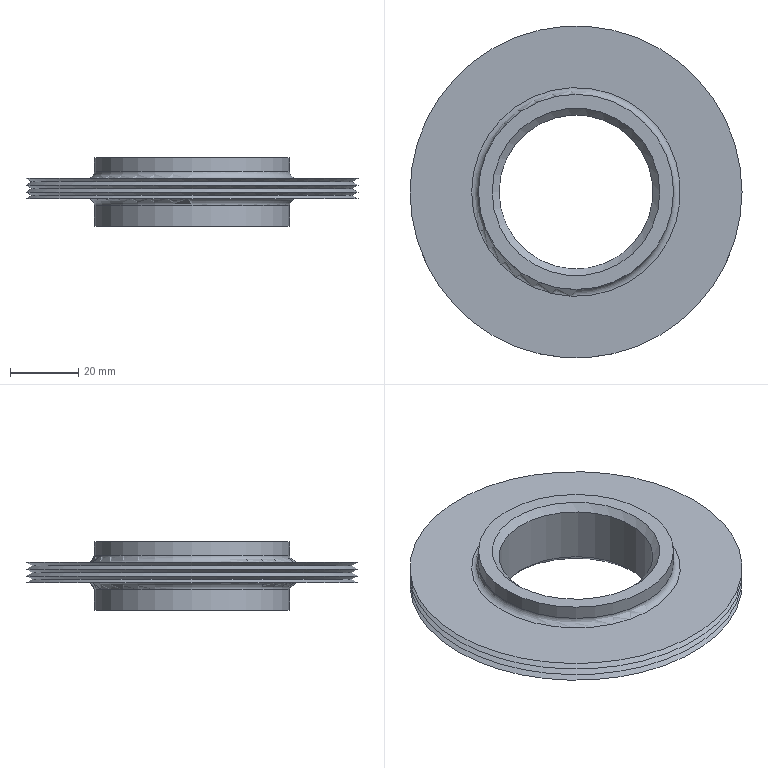Part | NX | features DATUM_CSYS 2, SKETCH 1, SWP104 1 | 1 solid | 17 faces | box 97 x 97 x 20 mm | volume 46420 mm3 | cone 8 | plane 4 | cylinder 3 | torus 2 | commonest cylinder face diameters 57 x2 45 x1
STEP:
#1=CARTESIAN_POINT('',(-48.5,0.,8.));
#2=VERTEX_POINT('',#1);
#3=CARTESIAN_POINT('',(0.,0.,8.));
#4=DIRECTION('',(0.,0.,-1.));
#5=DIRECTION('',(-1.,0.,0.));
#6=AXIS2_PLACEMENT_3D('',#3,#4,#5);
#7=CIRCLE('',#6,48.5);
#8=EDGE_CURVE('',#2,#2,#7,.T.);
#9=ORIENTED_EDGE('',*,*,#8,.F.);
#10=EDGE_LOOP('',(#9));
#11=FACE_BOUND('',#10,.T.);
#12=CARTESIAN_POINT('',(-46.768,0.,9.));
#13=VERTEX_POINT('',#12);
#14=CARTESIAN_POINT('',(0.,0.,9.));
#15=DIRECTION('',(0.,0.,-1.));
#16=DIRECTION('',(-1.,0.,0.));
#17=AXIS2_PLACEMENT_3D('',#14,#15,#16);
#18=CIRCLE('',#17,46.768);
#19=EDGE_CURVE('',#13,#13,#18,.T.);
#20=ORIENTED_EDGE('',*,*,#19,.T.);
#21=EDGE_LOOP('',(#20));
#22=FACE_BOUND('',#21,.T.);
#23=CARTESIAN_POINT('',(0.,0.,9.));
#24=DIRECTION('',(0.,0.,-1.));
#25=DIRECTION('',(-1.,0.,0.));
#26=AXIS2_PLACEMENT_3D('',#23,#24,#25);
#27=CONICAL_SURFACE('',#26,46.768,1.047);
#28=ADVANCED_FACE('',(#11,#22),#27,.T.);
#29=CARTESIAN_POINT('',(-30.5,0.,8.));
#30=VERTEX_POINT('',#29);
#31=CARTESIAN_POINT('',(0.,0.,8.));
#32=DIRECTION('',(0.,0.,-1.));
#33=DIRECTION('',(-1.,0.,0.));
#34=AXIS2_PLACEMENT_3D('',#31,#32,#33);
#35=CIRCLE('',#34,30.5);
#36=EDGE_CURVE('',#30,#30,#35,.T.);
#37=ORIENTED_EDGE('',*,*,#36,.F.);
#38=EDGE_LOOP('',(#37));
#39=FACE_BOUND('',#38,.T.);
#40=ORIENTED_EDGE('',*,*,#8,.T.);
#41=EDGE_LOOP('',(#40));
#42=FACE_BOUND('',#41,.T.);
#43=CARTESIAN_POINT('',(0.,-48.5,8.));
#44=DIRECTION('',(0.,0.,1.));
#45=DIRECTION('',(1.,0.,0.));
#46=AXIS2_PLACEMENT_3D('',#43,#44,#45);
#47=PLANE('',#46);
#48=ADVANCED_FACE('',(#39,#42),#47,.F.);
#49=CARTESIAN_POINT('',(-28.5,0.,6.));
#50=VERTEX_POINT('',#49);
#51=CARTESIAN_POINT('',(0.,0.,6.));
#52=DIRECTION('',(0.,0.,-1.));
#53=DIRECTION('',(-1.,0.,0.));
#54=AXIS2_PLACEMENT_3D('',#51,#52,#53);
#55=CIRCLE('',#54,28.5);
#56=EDGE_CURVE('',#50,#50,#55,.T.);
#57=ORIENTED_EDGE('',*,*,#56,.F.);
#58=EDGE_LOOP('',(#57));
#59=FACE_BOUND('',#58,.T.);
#60=ORIENTED_EDGE('',*,*,#36,.T.);
#61=EDGE_LOOP('',(#60));
#62=FACE_BOUND('',#61,.T.);
#63=CARTESIAN_POINT('',(0.,0.,6.));
#64=DIRECTION('',(0.,0.,-1.));
#65=DIRECTION('',(-1.,0.,0.));
#66=AXIS2_PLACEMENT_3D('',#63,#64,#65);
#67=TOROIDAL_SURFACE('',#66,30.5,2.);
#68=ADVANCED_FACE('',(#59,#62),#67,.F.);
#69=CARTESIAN_POINT('',(-28.5,0.,0.));
#70=VERTEX_POINT('',#69);
#71=CARTESIAN_POINT('',(0.,0.,0.));
#72=DIRECTION('',(0.,0.,-1.));
#73=DIRECTION('',(-1.,0.,0.));
#74=AXIS2_PLACEMENT_3D('',#71,#72,#73);
#75=CIRCLE('',#74,28.5);
#76=EDGE_CURVE('',#70,#70,#75,.T.);
#77=ORIENTED_EDGE('',*,*,#76,.F.);
#78=EDGE_LOOP('',(#77));
#79=FACE_BOUND('',#78,.T.);
#80=ORIENTED_EDGE('',*,*,#56,.T.);
#81=EDGE_LOOP('',(#80));
#82=FACE_BOUND('',#81,.T.);
#83=CARTESIAN_POINT('',(0.,0.,0.));
#84=DIRECTION('',(0.,0.,-1.));
#85=DIRECTION('',(-1.,0.,0.));
#86=AXIS2_PLACEMENT_3D('',#83,#84,#85);
#87=CYLINDRICAL_SURFACE('',#86,28.5);
#88=ADVANCED_FACE('',(#79,#82),#87,.T.);
#89=CARTESIAN_POINT('',(-24.5,0.,0.));
#90=VERTEX_POINT('',#89);
#91=CARTESIAN_POINT('',(0.,0.,0.));
#92=DIRECTION('',(0.,0.,-1.));
#93=DIRECTION('',(-1.,0.,0.));
#94=AXIS2_PLACEMENT_3D('',#91,#92,#93);
#95=CIRCLE('',#94,24.5);
#96=EDGE_CURVE('',#90,#90,#95,.T.);
#97=ORIENTED_EDGE('',*,*,#96,.F.);
#98=EDGE_LOOP('',(#97));
#99=FACE_BOUND('',#98,.T.);
#100=ORIENTED_EDGE('',*,*,#76,.T.);
#101=EDGE_LOOP('',(#100));
#102=FACE_BOUND('',#101,.T.);
#103=CARTESIAN_POINT('',(0.,-28.5,0.));
#104=DIRECTION('',(0.,0.,1.));
#105=DIRECTION('',(1.,0.,0.));
#106=AXIS2_PLACEMENT_3D('',#103,#104,#105);
#107=PLANE('',#106);
#108=ADVANCED_FACE('',(#99,#102),#107,.F.);
#109=CARTESIAN_POINT('',(-22.5,0.,2.));
#110=VERTEX_POINT('',#109);
#111=CARTESIAN_POINT('',(0.,0.,2.));
#112=DIRECTION('',(0.,0.,-1.));
#113=DIRECTION('',(-1.,0.,0.));
#114=AXIS2_PLACEMENT_3D('',#111,#112,#113);
#115=CIRCLE('',#114,22.5);
#116=EDGE_CURVE('',#110,#110,#115,.T.);
#117=ORIENTED_EDGE('',*,*,#116,.F.);
#118=EDGE_LOOP('',(#117));
#119=FACE_BOUND('',#118,.T.);
#120=ORIENTED_EDGE('',*,*,#96,.T.);
#121=EDGE_LOOP('',(#120));
#122=FACE_BOUND('',#121,.T.);
#123=CARTESIAN_POINT('',(0.,0.,0.));
#124=DIRECTION('',(0.,0.,-1.));
#125=DIRECTION('',(-1.,0.,0.));
#126=AXIS2_PLACEMENT_3D('',#123,#124,#125);
#127=CONICAL_SURFACE('',#126,24.5,0.7854);
#128=ADVANCED_FACE('',(#119,#122),#127,.F.);
#129=CARTESIAN_POINT('',(-22.5,0.,18.));
#130=VERTEX_POINT('',#129);
#131=CARTESIAN_POINT('',(0.,0.,18.));
#132=DIRECTION('',(0.,0.,-1.));
#133=DIRECTION('',(-1.,0.,0.));
#134=AXIS2_PLACEMENT_3D('',#131,#132,#133);
#135=CIRCLE('',#134,22.5);
#136=EDGE_CURVE('',#130,#130,#135,.T.);
#137=ORIENTED_EDGE('',*,*,#136,.F.);
#138=EDGE_LOOP('',(#137));
#139=FACE_BOUND('',#138,.T.);
#140=ORIENTED_EDGE('',*,*,#116,.T.);
#141=EDGE_LOOP('',(#140));
#142=FACE_BOUND('',#141,.T.);
#143=CARTESIAN_POINT('',(0.,0.,0.));
#144=DIRECTION('',(0.,0.,-1.));
#145=DIRECTION('',(-1.,0.,0.));
#146=AXIS2_PLACEMENT_3D('',#143,#144,#145);
#147=CYLINDRICAL_SURFACE('',#146,22.5);
#148=ADVANCED_FACE('',(#139,#142),#147,.F.);
#149=CARTESIAN_POINT('',(-24.5,0.,20.));
#150=VERTEX_POINT('',#149);
#151=CARTESIAN_POINT('',(0.,0.,20.));
#152=DIRECTION('',(0.,0.,-1.));
#153=DIRECTION('',(-1.,0.,0.));
#154=AXIS2_PLACEMENT_3D('',#151,#152,#153);
#155=CIRCLE('',#154,24.5);
#156=EDGE_CURVE('',#150,#150,#155,.T.);
#157=ORIENTED_EDGE('',*,*,#156,.F.);
#158=EDGE_LOOP('',(#157));
#159=FACE_BOUND('',#158,.T.);
#160=ORIENTED_EDGE('',*,*,#136,.T.);
#161=EDGE_LOOP('',(#160));
#162=FACE_BOUND('',#161,.T.);
#163=CARTESIAN_POINT('',(0.,0.,18.));
#164=DIRECTION('',(0.,0.,1.));
#165=DIRECTION('',(1.,0.,0.));
#166=AXIS2_PLACEMENT_3D('',#163,#164,#165);
#167=CONICAL_SURFACE('',#166,22.5,0.7854);
#168=ADVANCED_FACE('',(#159,#162),#167,.F.);
#169=CARTESIAN_POINT('',(-28.5,0.,20.));
#170=VERTEX_POINT('',#169);
#171=CARTESIAN_POINT('',(0.,0.,20.));
#172=DIRECTION('',(0.,0.,-1.));
#173=DIRECTION('',(-1.,0.,0.));
#174=AXIS2_PLACEMENT_3D('',#171,#172,#173);
#175=CIRCLE('',#174,28.5);
#176=EDGE_CURVE('',#170,#170,#175,.T.);
#177=ORIENTED_EDGE('',*,*,#176,.F.);
#178=EDGE_LOOP('',(#177));
#179=FACE_BOUND('',#178,.T.);
#180=ORIENTED_EDGE('',*,*,#156,.T.);
#181=EDGE_LOOP('',(#180));
#182=FACE_BOUND('',#181,.T.);
#183=CARTESIAN_POINT('',(0.,-24.5,20.));
#184=DIRECTION('',(0.,0.,-1.));
#185=DIRECTION('',(-1.,0.,0.));
#186=AXIS2_PLACEMENT_3D('',#183,#184,#185);
#187=PLANE('',#186);
#188=ADVANCED_FACE('',(#179,#182),#187,.F.);
#189=CARTESIAN_POINT('',(-28.5,0.,16.));
#190=VERTEX_POINT('',#189);
#191=CARTESIAN_POINT('',(0.,0.,16.));
#192=DIRECTION('',(0.,0.,-1.));
#193=DIRECTION('',(-1.,0.,0.));
#194=AXIS2_PLACEMENT_3D('',#191,#192,#193);
#195=CIRCLE('',#194,28.5);
#196=EDGE_CURVE('',#190,#190,#195,.T.);
#197=ORIENTED_EDGE('',*,*,#196,.F.);
#198=EDGE_LOOP('',(#197));
#199=FACE_BOUND('',#198,.T.);
#200=ORIENTED_EDGE('',*,*,#176,.T.);
#201=EDGE_LOOP('',(#200));
#202=FACE_BOUND('',#201,.T.);
#203=CARTESIAN_POINT('',(0.,0.,0.));
#204=DIRECTION('',(0.,0.,-1.));
#205=DIRECTION('',(-1.,0.,0.));
#206=AXIS2_PLACEMENT_3D('',#203,#204,#205);
#207=CYLINDRICAL_SURFACE('',#206,28.5);
#208=ADVANCED_FACE('',(#199,#202),#207,.T.);
#209=CARTESIAN_POINT('',(-30.5,0.,14.));
#210=VERTEX_POINT('',#209);
#211=CARTESIAN_POINT('',(0.,0.,14.));
#212=DIRECTION('',(0.,0.,-1.));
#213=DIRECTION('',(-1.,0.,0.));
#214=AXIS2_PLACEMENT_3D('',#211,#212,#213);
#215=CIRCLE('',#214,30.5);
#216=EDGE_CURVE('',#210,#210,#215,.T.);
#217=ORIENTED_EDGE('',*,*,#216,.F.);
#218=EDGE_LOOP('',(#217));
#219=FACE_BOUND('',#218,.T.);
#220=ORIENTED_EDGE('',*,*,#196,.T.);
#221=EDGE_LOOP('',(#220));
#222=FACE_BOUND('',#221,.T.);
#223=CARTESIAN_POINT('',(0.,0.,16.));
#224=DIRECTION('',(0.,0.,-1.));
#225=DIRECTION('',(-1.,0.,0.));
#226=AXIS2_PLACEMENT_3D('',#223,#224,#225);
#227=TOROIDAL_SURFACE('',#226,30.5,2.);
#228=ADVANCED_FACE('',(#219,#222),#227,.F.);
#229=CARTESIAN_POINT('',(-48.5,0.,14.));
#230=VERTEX_POINT('',#229);
#231=CARTESIAN_POINT('',(0.,0.,14.));
#232=DIRECTION('',(0.,0.,-1.));
#233=DIRECTION('',(-1.,0.,0.));
#234=AXIS2_PLACEMENT_3D('',#231,#232,#233);
#235=CIRCLE('',#234,48.5);
#236=EDGE_CURVE('',#230,#230,#235,.T.);
#237=ORIENTED_EDGE('',*,*,#236,.F.);
#238=EDGE_LOOP('',(#237));
#239=FACE_BOUND('',#238,.T.);
#240=ORIENTED_EDGE('',*,*,#216,.T.);
#241=EDGE_LOOP('',(#240));
#242=FACE_BOUND('',#241,.T.);
#243=CARTESIAN_POINT('',(0.,-30.5,14.));
#244=DIRECTION('',(0.,0.,-1.));
#245=DIRECTION('',(-1.,0.,0.));
#246=AXIS2_PLACEMENT_3D('',#243,#244,#245);
#247=PLANE('',#246);
#248=ADVANCED_FACE('',(#239,#242),#247,.F.);
#249=CARTESIAN_POINT('',(-46.768,0.,13.));
#250=VERTEX_POINT('',#249);
#251=CARTESIAN_POINT('',(0.,0.,13.));
#252=DIRECTION('',(0.,0.,-1.));
#253=DIRECTION('',(-1.,0.,0.));
#254=AXIS2_PLACEMENT_3D('',#251,#252,#253);
#255=CIRCLE('',#254,46.768);
#256=EDGE_CURVE('',#250,#250,#255,.T.);
#257=ORIENTED_EDGE('',*,*,#256,.F.);
#258=EDGE_LOOP('',(#257));
#259=FACE_BOUND('',#258,.T.);
#260=ORIENTED_EDGE('',*,*,#236,.T.);
#261=EDGE_LOOP('',(#260));
#262=FACE_BOUND('',#261,.T.);
#263=CARTESIAN_POINT('',(0.,0.,14.));
#264=DIRECTION('',(0.,0.,1.));
#265=DIRECTION('',(1.,0.,0.));
#266=AXIS2_PLACEMENT_3D('',#263,#264,#265);
#267=CONICAL_SURFACE('',#266,48.5,1.047);
#268=ADVANCED_FACE('',(#259,#262),#267,.T.);
#269=CARTESIAN_POINT('',(-48.5,0.,12.));
#270=VERTEX_POINT('',#269);
#271=CARTESIAN_POINT('',(0.,0.,12.));
#272=DIRECTION('',(0.,0.,-1.));
#273=DIRECTION('',(-1.,0.,0.));
#274=AXIS2_PLACEMENT_3D('',#271,#272,#273);
#275=CIRCLE('',#274,48.5);
#276=EDGE_CURVE('',#270,#270,#275,.T.);
#277=ORIENTED_EDGE('',*,*,#276,.F.);
#278=EDGE_LOOP('',(#277));
#279=FACE_BOUND('',#278,.T.);
#280=ORIENTED_EDGE('',*,*,#256,.T.);
#281=EDGE_LOOP('',(#280));
#282=FACE_BOUND('',#281,.T.);
#283=CARTESIAN_POINT('',(0.,0.,13.));
#284=DIRECTION('',(0.,0.,-1.));
#285=DIRECTION('',(-1.,0.,0.));
#286=AXIS2_PLACEMENT_3D('',#283,#284,#285);
#287=CONICAL_SURFACE('',#286,46.768,1.047);
#288=ADVANCED_FACE('',(#279,#282),#287,.T.);
#289=CARTESIAN_POINT('',(-46.768,0.,11.));
#290=VERTEX_POINT('',#289);
#291=CARTESIAN_POINT('',(0.,0.,11.));
#292=DIRECTION('',(0.,0.,-1.));
#293=DIRECTION('',(-1.,0.,0.));
#294=AXIS2_PLACEMENT_3D('',#291,#292,#293);
#295=CIRCLE('',#294,46.768);
#296=EDGE_CURVE('',#290,#290,#295,.T.);
#297=ORIENTED_EDGE('',*,*,#296,.F.);
#298=EDGE_LOOP('',(#297));
#299=FACE_BOUND('',#298,.T.);
#300=ORIENTED_EDGE('',*,*,#276,.T.);
#301=EDGE_LOOP('',(#300));
#302=FACE_BOUND('',#301,.T.);
#303=CARTESIAN_POINT('',(0.,0.,12.));
#304=DIRECTION('',(0.,0.,1.));
#305=DIRECTION('',(1.,0.,0.));
#306=AXIS2_PLACEMENT_3D('',#303,#304,#305);
#307=CONICAL_SURFACE('',#306,48.5,1.047);
#308=ADVANCED_FACE('',(#299,#302),#307,.T.);
#309=CARTESIAN_POINT('',(-48.5,0.,10.));
#310=VERTEX_POINT('',#309);
#311=CARTESIAN_POINT('',(0.,0.,10.));
#312=DIRECTION('',(0.,0.,-1.));
#313=DIRECTION('',(-1.,0.,0.));
#314=AXIS2_PLACEMENT_3D('',#311,#312,#313);
#315=CIRCLE('',#314,48.5);
#316=EDGE_CURVE('',#310,#310,#315,.T.);
#317=ORIENTED_EDGE('',*,*,#316,.F.);
#318=EDGE_LOOP('',(#317));
#319=FACE_BOUND('',#318,.T.);
#320=ORIENTED_EDGE('',*,*,#296,.T.);
#321=EDGE_LOOP('',(#320));
#322=FACE_BOUND('',#321,.T.);
#323=CARTESIAN_POINT('',(0.,0.,11.));
#324=DIRECTION('',(0.,0.,-1.));
#325=DIRECTION('',(-1.,0.,0.));
#326=AXIS2_PLACEMENT_3D('',#323,#324,#325);
#327=CONICAL_SURFACE('',#326,46.768,1.047);
#328=ADVANCED_FACE('',(#319,#322),#327,.T.);
#329=ORIENTED_EDGE('',*,*,#19,.F.);
#330=EDGE_LOOP('',(#329));
#331=FACE_BOUND('',#330,.T.);
#332=ORIENTED_EDGE('',*,*,#316,.T.);
#333=EDGE_LOOP('',(#332));
#334=FACE_BOUND('',#333,.T.);
#335=CARTESIAN_POINT('',(0.,0.,10.));
#336=DIRECTION('',(0.,0.,1.));
#337=DIRECTION('',(1.,0.,0.));
#338=AXIS2_PLACEMENT_3D('',#335,#336,#337);
#339=CONICAL_SURFACE('',#338,48.5,1.047);
#340=ADVANCED_FACE('',(#331,#334),#339,.T.);
#341=CLOSED_SHELL('',(#28,#48,#68,#88,#108,#128,#148,#168,#188,#208,#228,#248,#268,#288,#308,#328,#340));
#342=MANIFOLD_SOLID_BREP('',#341);
#343=(LENGTH_UNIT()NAMED_UNIT(*)SI_UNIT(.MILLI.,.METRE.));
#344=UNCERTAINTY_MEASURE_WITH_UNIT(LENGTH_MEASURE(0.00001),#343,'','');
#345=(NAMED_UNIT(*)PLANE_ANGLE_UNIT()SI_UNIT($,.RADIAN.));
#346=(NAMED_UNIT(*)SI_UNIT($,.STERADIAN.)SOLID_ANGLE_UNIT());
#347=(GEOMETRIC_REPRESENTATION_CONTEXT(3)GLOBAL_UNCERTAINTY_ASSIGNED_CONTEXT((#344))GLOBAL_UNIT_ASSIGNED_CONTEXT((#343,#345,#346))REPRESENTATION_CONTEXT('',''));
#348=ADVANCED_BREP_SHAPE_REPRESENTATION('',(#342),#347);